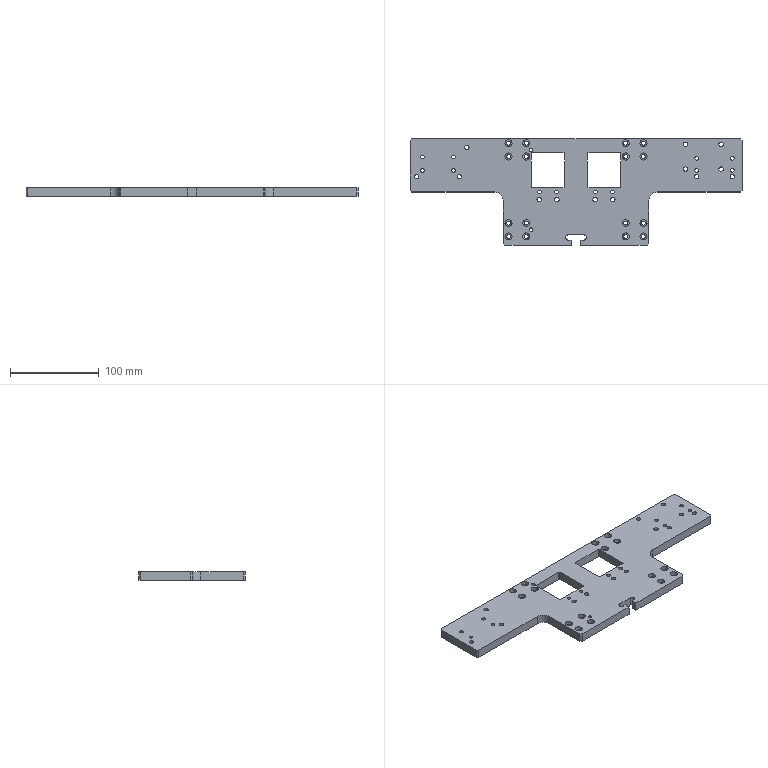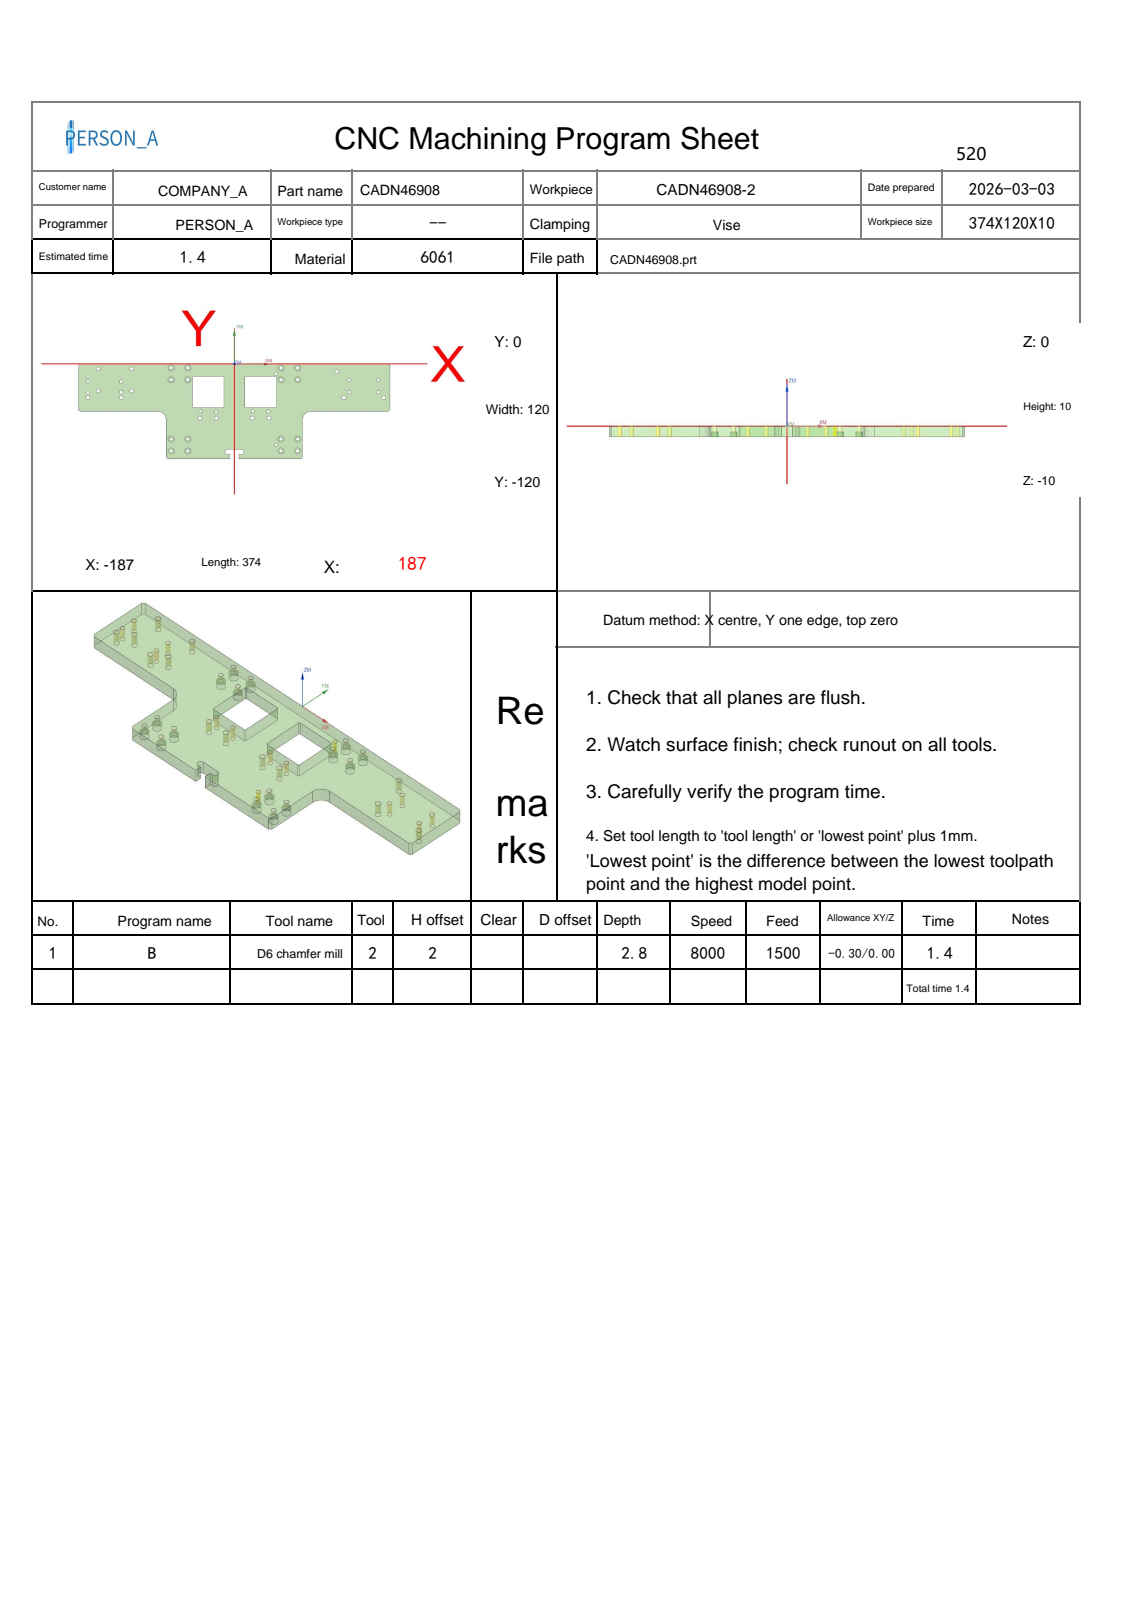NC program | NX | posted by the shop | part box 374 x 120 x 10 mm
Whole program:
%
O0001
(Machine time: 1.56 MIN)
(===Total Tool:1===)
(T2=D6 chamfer mill   D=6.   R=0.   D-  H02 Z=-2.8  )
G80 G90 G17 G49 G40
G91 G28 Z0
M01
N1 T02 M06
(D6 chamfer mill  D=6. R=0. H=02 ce=-0.30 di=0.00)
G00 G90 G54 X40.358 Y-54.3 M03 S7000
G43 H02 Z50.
M08
Z2.5
G01 X49.543 Z-.843 F1500.
X49.635 Y-54.271 Z-.878
X49.714 Y-54.214 Z-.914
X49.771 Y-54.135 Z-.949
X49.8 Y-54.043 Z-.985
Y-54. Z-1.
Y-17.
G03 X49.5 Y-16.7 I-.3 J0.0
G01 X13.5
G03 X13.2 Y-17. I0.0 J-.3
G01 Y-54.
G03 X13.5 Y-54.3 I.3 J0.0
G01 X49.5
G03 X49.8 Y-54. I0.0 J.3
G01 Y-53.5
Z1.5
G00 Z50.
X13.843 Y-120.7
Z2.5
G01 X5.722 Z-.456
X5.523 Y-120.664 Z-.529
X5.335 Y-120.589 Z-.603
X5.166 Y-120.477 Z-.677
X5.023 Y-120.334 Z-.751
X4.911 Y-120.165 Z-.824
X4.836 Y-119.977 Z-.898
X4.8 Y-119.778 Z-.972
Y-119.7 Z-1.
Y-114.5
G02 X5.8 Y-113.5 I1. J0.0
G01 X8.5
G03 X10.8 Y-111.2 I0.0 J2.3
X8.5 Y-108.9 I-2.3 J0.0
G01 X-8.5
G03 X-10.8 Y-111.2 I0.0 J-2.3
X-8.5 Y-113.5 I2.3 J0.0
G01 X-5.8
G02 X-4.8 Y-114.5 I0.0 J-1.
G01 Y-119.7
G02 X-5.8 Y-120.7 I-1. J0.0
G01 X-79.876
G02 X-80.583 Y-120.407 I0.0 J1.
G01 X-82.407 Y-118.583
G02 X-82.7 Y-117.876 I.707 J.707
G01 Y-70.
G03 X-92. Y-60.7 I-9.3 J0.0
G01 X-184.876
G02 X-185.583 Y-60.407 I0.0 J1.
G01 X-187.407 Y-58.583
G02 X-187.7 Y-57.876 I.707 J.707
G01 Y-2.124
G02 X-187.407 Y-1.417 I1. J0.0
G01 X-185.583 Y.407
G02 X-184.876 Y.7 I.707 J-.707
G01 X184.876
G02 X185.583 Y.407 I0.0 J-1.
G01 X187.407 Y-1.417
G02 X187.7 Y-2.124 I-.707 J-.707
G01 Y-57.876
G02 X187.407 Y-58.583 I-1. J0.0
G01 X185.583 Y-60.407
G02 X184.876 Y-60.7 I-.707 J.707
G01 X92.
G03 X82.7 Y-70. I0.0 J-9.3
G01 Y-117.876
G02 X82.407 Y-118.583 I-1. J0.0
G01 X80.583 Y-120.407
G02 X79.876 Y-120.7 I-.707 J.707
G01 X5.8
G02 X4.8 Y-119.7 I0.0 J1.
G01 Y-119.2
Z1.5
G00 Z50.
X-22.642 Y-54.3
Z2.5
G01 X-13.457 Z-.843
X-13.365 Y-54.271 Z-.878
X-13.286 Y-54.214 Z-.914
X-13.229 Y-54.135 Z-.949
X-13.2 Y-54.043 Z-.985
Y-54. Z-1.
Y-17.
G03 X-13.5 Y-16.7 I-.3 J0.0
G01 X-49.5
G03 X-49.8 Y-17. I0.0 J-.3
G01 Y-54.
G03 X-49.5 Y-54.3 I.3 J0.0
G01 X-13.5
G03 X-13.2 Y-54. I0.0 J.3
G01 Y-53.5
Z1.5
G00 Z50.
G00 G90 X50.5 Y-12.5 M03 S8000
Z50.
G98 G81 X50.5 Y-12.5 Z-2.3 R3. F1000.
Y-102.5
G80
G00 Z50.
G00 G90 X-56. Y-95. M03 S8000
Z50.
G98 G81 X-56. Y-95. Z-2.55 R3. F1000.
Y-110.
X-76.
Y-95.
Y-20.
Y-5.
X-56.
Y-20.
X56.
Y-5.
X76.
Y-20.
Y-95.
Y-110.
X56.
Y-95.
G80
G00 Z50.
G00 G90 X179.471 Y-42.7 M03 S8000
Z50.
G98 G81 X179.471 Y-42.7 Z-2.8 R3. F1000.
X131.471
X122.971 Y-9.6
X41.5 Y-68.5
X21.5
X-21.5
X-41.5
X-136. Y-42.7
X-123.5 Y-34.2
Y-6.2
X-163.5
Y-34.2
X-176. Y-42.7
G80
G00 Z50.
G00 G90 X172.971 Y-35.7 M03 S8000
Z50.
G98 G81 X172.971 Y-35.7 Z-2.7 R3. F1000.
Y-20.7
X137.971
Y-35.7
X41. Y-60.
X22.
X-22.
X-41.
X-136. Y-35.7
Y-22.2
X-176.
Y-35.7
G80
G00 Z50.
M05
M09
G91 G28 Z0.0
G91 G28 Y0.0
M30
%